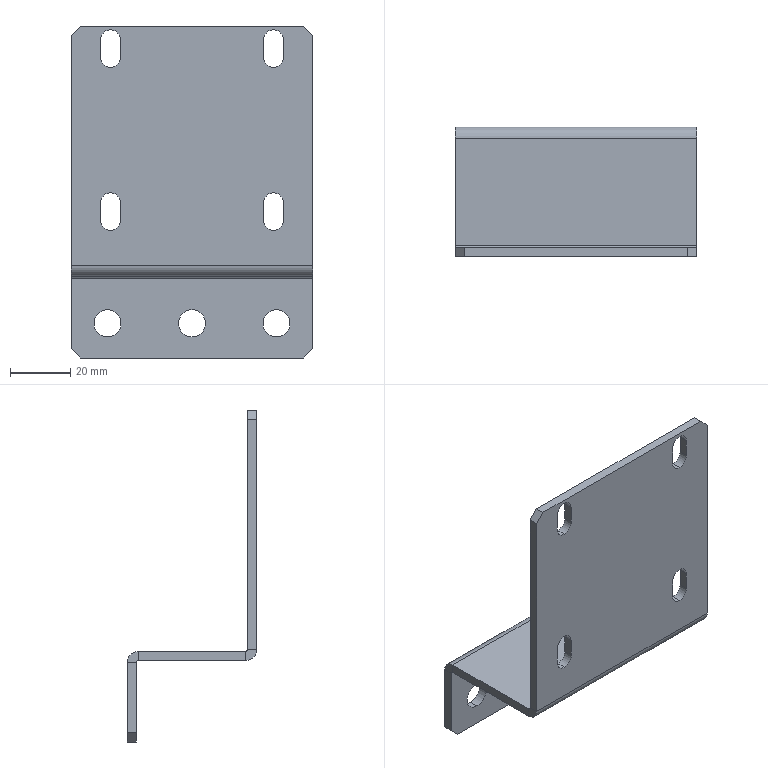Part | STEP file | 1 solid | 52 faces | box 80 x 43 x 110 mm | volume 34046 mm3 | plane 30 | cylinder 22 | commonest cylinder face diameters 6.5 x12 9 x6 1.473 x2 7.473 x2